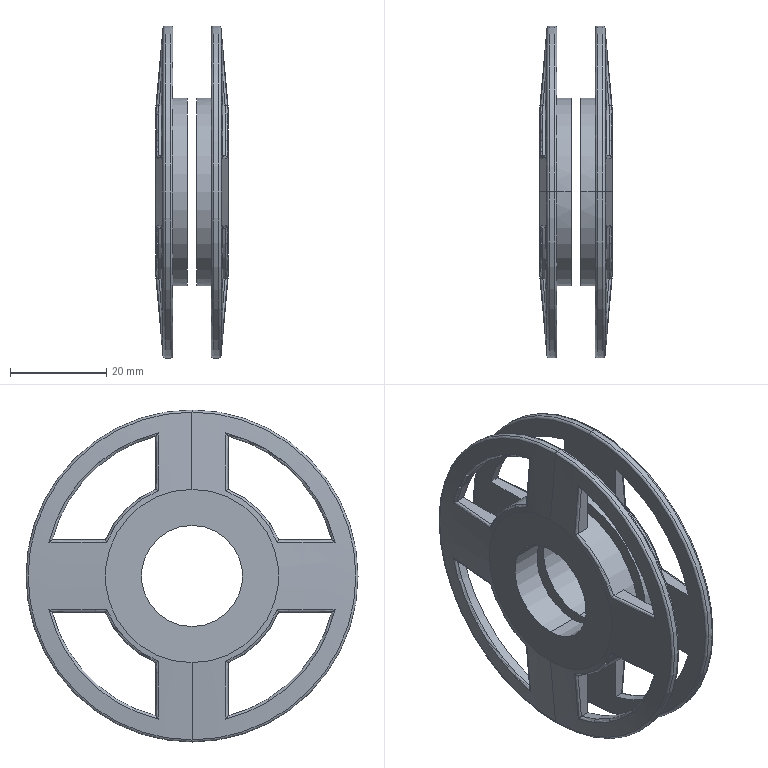Part | STEP file | Plastic cage for metal toothed Idler | 2 solids | 86 faces | box 15 x 69 x 69 mm | volume 18640 mm3 | torus 24 | plane 22 | cylinder 20 | spline 16 | cone 4 | commonest cylinder face diameters 60 x8 21 x4 39 x4 69 x4